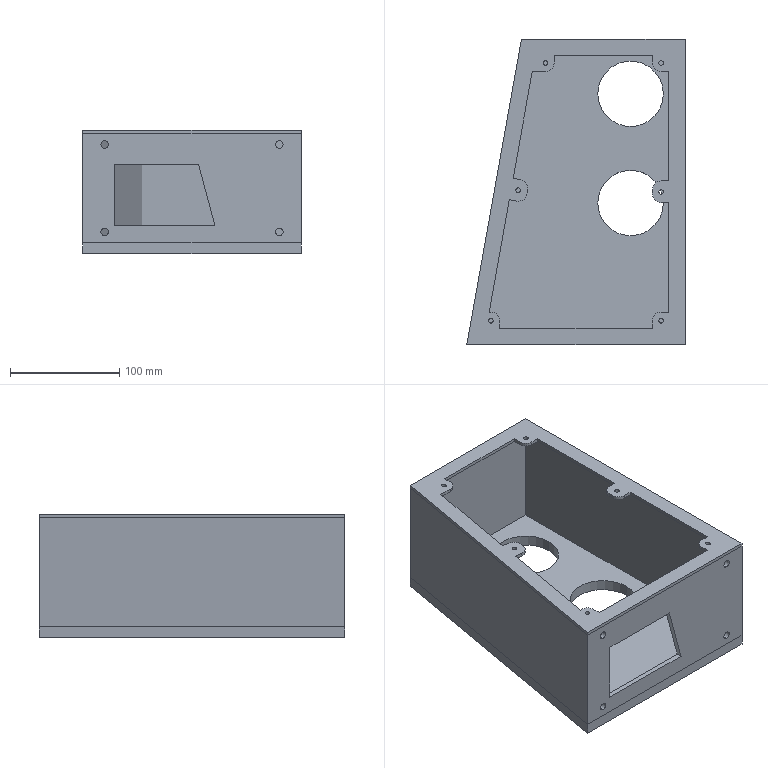Part | STEP file | Drive box QY-1-01 | 3 solids | 84 faces | box 200 x 280 x 113 mm | volume 897718 mm3 | plane 46 | cylinder 38 | commonest cylinder face diameters 4.2 x12 6.8 x8 16 x8 5 x4 60 x4 12.5 x2